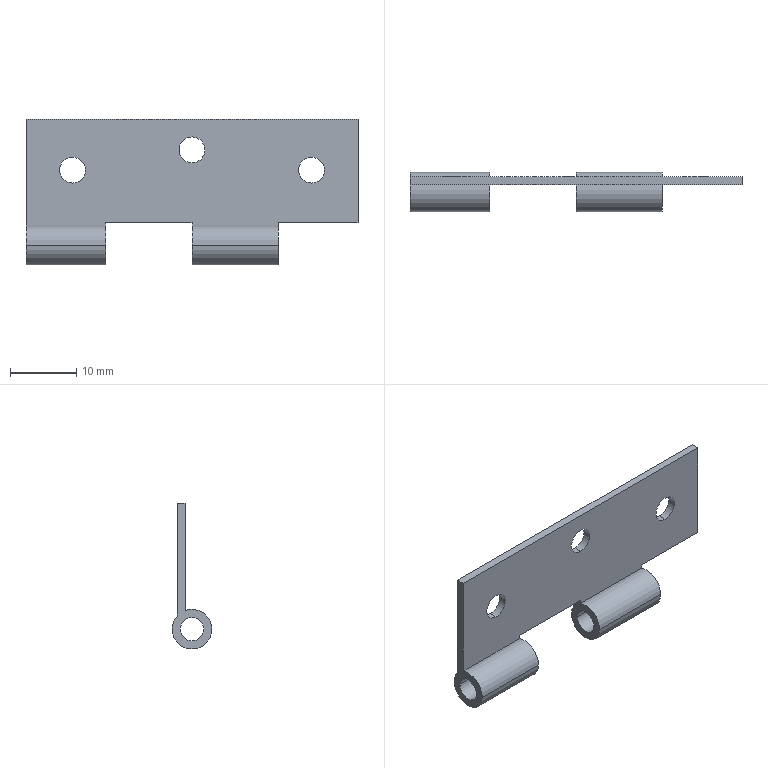Part | SolidWorks | features BaseBody 1 | 1 solid | 29 faces | box 50 x 6 x 22 mm | volume 1387 mm3 | cylinder 19 | plane 10 | commonest cylinder face diameters 3.9 x9 6 x6 3.5 x4
STEP:
#1=CARTESIAN_POINT('',(-595.131,801.497,187.232));
#2=VERTEX_POINT('',#1);
#3=CARTESIAN_POINT('',(-593.181,801.497,185.282));
#4=VERTEX_POINT('',#3);
#5=CARTESIAN_POINT('',(-595.131,801.497,185.282));
#6=DIRECTION('',(0.,1.,0.));
#7=DIRECTION('',(0.,0.,1.));
#8=AXIS2_PLACEMENT_3D('',#5,#6,#7);
#9=CIRCLE('',#8,1.95);
#10=EDGE_CURVE('',#2,#4,#9,.T.);
#11=ORIENTED_EDGE('',*,*,#10,.T.);
#12=CARTESIAN_POINT('',(-593.181,800.297,185.282));
#13=VERTEX_POINT('',#12);
#14=CARTESIAN_POINT('',(-593.181,850.297,185.282));
#15=DIRECTION('',(0.,-1.,0.));
#16=VECTOR('',#15,1000.);
#17=LINE('',#14,#16);
#18=EDGE_CURVE('',#4,#13,#17,.T.);
#19=ORIENTED_EDGE('',*,*,#18,.T.);
#20=CARTESIAN_POINT('',(-595.131,800.297,187.232));
#21=VERTEX_POINT('',#20);
#22=CARTESIAN_POINT('',(-595.131,800.297,185.282));
#23=DIRECTION('',(0.,-1.,0.));
#24=DIRECTION('',(0.,0.,-1.));
#25=AXIS2_PLACEMENT_3D('',#22,#23,#24);
#26=CIRCLE('',#25,1.95);
#27=EDGE_CURVE('',#13,#21,#26,.T.);
#28=ORIENTED_EDGE('',*,*,#27,.T.);
#29=CARTESIAN_POINT('',(-595.131,801.497,187.232));
#30=DIRECTION('',(0.,-1.,0.));
#31=VECTOR('',#30,1000.);
#32=LINE('',#29,#31);
#33=EDGE_CURVE('',#2,#21,#32,.T.);
#34=ORIENTED_EDGE('',*,*,#33,.F.);
#35=EDGE_LOOP('',(#11,#19,#28,#34));
#36=FACE_OUTER_BOUND('',#35,.T.);
#37=CARTESIAN_POINT('',(-595.131,850.297,185.282));
#38=DIRECTION('',(0.,-1.,0.));
#39=DIRECTION('',(1.,0.,0.));
#40=AXIS2_PLACEMENT_3D('',#37,#38,#39);
#41=CYLINDRICAL_SURFACE('',#40,1.95);
#42=ADVANCED_FACE('',(#36),#41,.F.);
#43=CARTESIAN_POINT('',(-631.131,801.497,187.232));
#44=VERTEX_POINT('',#43);
#45=CARTESIAN_POINT('',(-629.181,801.497,185.282));
#46=VERTEX_POINT('',#45);
#47=CARTESIAN_POINT('',(-631.131,801.497,185.282));
#48=DIRECTION('',(0.,1.,0.));
#49=DIRECTION('',(0.,0.,1.));
#50=AXIS2_PLACEMENT_3D('',#47,#48,#49);
#51=CIRCLE('',#50,1.95);
#52=EDGE_CURVE('',#44,#46,#51,.T.);
#53=ORIENTED_EDGE('',*,*,#52,.T.);
#54=CARTESIAN_POINT('',(-629.181,800.297,185.282));
#55=VERTEX_POINT('',#54);
#56=CARTESIAN_POINT('',(-629.181,850.297,185.282));
#57=DIRECTION('',(0.,-1.,0.));
#58=VECTOR('',#57,1000.);
#59=LINE('',#56,#58);
#60=EDGE_CURVE('',#46,#55,#59,.T.);
#61=ORIENTED_EDGE('',*,*,#60,.T.);
#62=CARTESIAN_POINT('',(-631.131,800.297,187.232));
#63=VERTEX_POINT('',#62);
#64=CARTESIAN_POINT('',(-631.131,800.297,185.282));
#65=DIRECTION('',(0.,-1.,0.));
#66=DIRECTION('',(0.,0.,-1.));
#67=AXIS2_PLACEMENT_3D('',#64,#65,#66);
#68=CIRCLE('',#67,1.95);
#69=EDGE_CURVE('',#55,#63,#68,.T.);
#70=ORIENTED_EDGE('',*,*,#69,.T.);
#71=CARTESIAN_POINT('',(-631.131,801.497,187.232));
#72=DIRECTION('',(0.,-1.,0.));
#73=VECTOR('',#72,1000.);
#74=LINE('',#71,#73);
#75=EDGE_CURVE('',#44,#63,#74,.T.);
#76=ORIENTED_EDGE('',*,*,#75,.F.);
#77=EDGE_LOOP('',(#53,#61,#70,#76));
#78=FACE_OUTER_BOUND('',#77,.T.);
#79=CARTESIAN_POINT('',(-631.131,850.297,185.282));
#80=DIRECTION('',(0.,-1.,0.));
#81=DIRECTION('',(1.,0.,0.));
#82=AXIS2_PLACEMENT_3D('',#79,#80,#81);
#83=CYLINDRICAL_SURFACE('',#82,1.95);
#84=ADVANCED_FACE('',(#78),#83,.F.);
#85=CARTESIAN_POINT('',(-613.131,801.497,190.282));
#86=VERTEX_POINT('',#85);
#87=CARTESIAN_POINT('',(-611.181,801.497,188.332));
#88=VERTEX_POINT('',#87);
#89=CARTESIAN_POINT('',(-613.131,801.497,188.332));
#90=DIRECTION('',(0.,1.,0.));
#91=DIRECTION('',(0.,0.,1.));
#92=AXIS2_PLACEMENT_3D('',#89,#90,#91);
#93=CIRCLE('',#92,1.95);
#94=EDGE_CURVE('',#86,#88,#93,.T.);
#95=ORIENTED_EDGE('',*,*,#94,.T.);
#96=CARTESIAN_POINT('',(-611.181,800.297,188.332));
#97=VERTEX_POINT('',#96);
#98=CARTESIAN_POINT('',(-611.181,850.297,188.332));
#99=DIRECTION('',(0.,-1.,0.));
#100=VECTOR('',#99,1000.);
#101=LINE('',#98,#100);
#102=EDGE_CURVE('',#88,#97,#101,.T.);
#103=ORIENTED_EDGE('',*,*,#102,.T.);
#104=CARTESIAN_POINT('',(-613.131,800.297,190.282));
#105=VERTEX_POINT('',#104);
#106=CARTESIAN_POINT('',(-613.131,800.297,188.332));
#107=DIRECTION('',(0.,-1.,0.));
#108=DIRECTION('',(1.,0.,0.));
#109=AXIS2_PLACEMENT_3D('',#106,#107,#108);
#110=CIRCLE('',#109,1.95);
#111=EDGE_CURVE('',#97,#105,#110,.T.);
#112=ORIENTED_EDGE('',*,*,#111,.T.);
#113=CARTESIAN_POINT('',(-613.131,800.297,190.282));
#114=DIRECTION('',(0.,1.,0.));
#115=VECTOR('',#114,1000.);
#116=LINE('',#113,#115);
#117=EDGE_CURVE('',#105,#86,#116,.T.);
#118=ORIENTED_EDGE('',*,*,#117,.T.);
#119=EDGE_LOOP('',(#95,#103,#112,#118));
#120=FACE_OUTER_BOUND('',#119,.T.);
#121=CARTESIAN_POINT('',(-613.131,850.297,188.332));
#122=DIRECTION('',(0.,-1.,0.));
#123=DIRECTION('',(1.,0.,0.));
#124=AXIS2_PLACEMENT_3D('',#121,#122,#123);
#125=CYLINDRICAL_SURFACE('',#124,1.95);
#126=ADVANCED_FACE('',(#120),#125,.F.);
#127=ORIENTED_EDGE('',*,*,#117,.F.);
#128=CARTESIAN_POINT('',(-613.131,800.297,186.382));
#129=VERTEX_POINT('',#128);
#130=CARTESIAN_POINT('',(-613.131,800.297,188.332));
#131=DIRECTION('',(0.,-1.,0.));
#132=DIRECTION('',(-1.,0.,0.));
#133=AXIS2_PLACEMENT_3D('',#130,#131,#132);
#134=CIRCLE('',#133,1.95);
#135=EDGE_CURVE('',#105,#129,#134,.T.);
#136=ORIENTED_EDGE('',*,*,#135,.T.);
#137=CARTESIAN_POINT('',(-613.131,801.497,186.382));
#138=VERTEX_POINT('',#137);
#139=CARTESIAN_POINT('',(-613.131,801.497,186.382));
#140=DIRECTION('',(0.,-1.,0.));
#141=VECTOR('',#140,1000.);
#142=LINE('',#139,#141);
#143=EDGE_CURVE('',#138,#129,#142,.T.);
#144=ORIENTED_EDGE('',*,*,#143,.F.);
#145=CARTESIAN_POINT('',(-613.131,801.497,188.332));
#146=DIRECTION('',(0.,1.,0.));
#147=DIRECTION('',(-1.,0.,0.));
#148=AXIS2_PLACEMENT_3D('',#145,#146,#147);
#149=CIRCLE('',#148,1.95);
#150=EDGE_CURVE('',#138,#86,#149,.T.);
#151=ORIENTED_EDGE('',*,*,#150,.T.);
#152=EDGE_LOOP('',(#127,#136,#144,#151));
#153=FACE_OUTER_BOUND('',#152,.T.);
#154=CARTESIAN_POINT('',(-613.131,850.297,188.332));
#155=DIRECTION('',(0.,-1.,0.));
#156=DIRECTION('',(1.,0.,0.));
#157=AXIS2_PLACEMENT_3D('',#154,#155,#156);
#158=CYLINDRICAL_SURFACE('',#157,1.95);
#159=ADVANCED_FACE('',(#153),#158,.F.);
#160=ORIENTED_EDGE('',*,*,#102,.F.);
#161=CARTESIAN_POINT('',(-613.131,801.497,188.332));
#162=DIRECTION('',(0.,1.,0.));
#163=DIRECTION('',(0.,0.,1.));
#164=AXIS2_PLACEMENT_3D('',#161,#162,#163);
#165=CIRCLE('',#164,1.95);
#166=EDGE_CURVE('',#88,#138,#165,.T.);
#167=ORIENTED_EDGE('',*,*,#166,.T.);
#168=ORIENTED_EDGE('',*,*,#143,.T.);
#169=CARTESIAN_POINT('',(-613.131,800.297,188.332));
#170=DIRECTION('',(0.,-1.,0.));
#171=DIRECTION('',(1.,0.,0.));
#172=AXIS2_PLACEMENT_3D('',#169,#170,#171);
#173=CIRCLE('',#172,1.95);
#174=EDGE_CURVE('',#129,#97,#173,.T.);
#175=ORIENTED_EDGE('',*,*,#174,.T.);
#176=EDGE_LOOP('',(#160,#167,#168,#175));
#177=FACE_OUTER_BOUND('',#176,.T.);
#178=CARTESIAN_POINT('',(-613.131,850.297,188.332));
#179=DIRECTION('',(0.,-1.,0.));
#180=DIRECTION('',(1.,0.,0.));
#181=AXIS2_PLACEMENT_3D('',#178,#179,#180);
#182=CYLINDRICAL_SURFACE('',#181,1.95);
#183=ADVANCED_FACE('',(#177),#182,.F.);
#184=CARTESIAN_POINT('',(-626.131,801.497,175.966));
#185=VERTEX_POINT('',#184);
#186=CARTESIAN_POINT('',(-626.131,801.497,177.382));
#187=VERTEX_POINT('',#186);
#188=CARTESIAN_POINT('',(-626.131,801.497,175.966));
#189=DIRECTION('',(0.,0.,1.));
#190=VECTOR('',#189,1000.);
#191=LINE('',#188,#190);
#192=EDGE_CURVE('',#185,#187,#191,.T.);
#193=ORIENTED_EDGE('',*,*,#192,.F.);
#194=CARTESIAN_POINT('',(-638.131,801.497,175.966));
#195=VERTEX_POINT('',#194);
#196=CARTESIAN_POINT('',(-626.131,801.497,175.966));
#197=DIRECTION('',(-1.,0.,0.));
#198=VECTOR('',#197,1000.);
#199=LINE('',#196,#198);
#200=EDGE_CURVE('',#185,#195,#199,.T.);
#201=ORIENTED_EDGE('',*,*,#200,.T.);
#202=CARTESIAN_POINT('',(-638.131,801.497,192.982));
#203=VERTEX_POINT('',#202);
#204=CARTESIAN_POINT('',(-638.131,801.497,192.982));
#205=DIRECTION('',(0.,0.,-1.));
#206=VECTOR('',#205,1000.);
#207=LINE('',#204,#206);
#208=EDGE_CURVE('',#203,#195,#207,.T.);
#209=ORIENTED_EDGE('',*,*,#208,.F.);
#210=CARTESIAN_POINT('',(-588.131,801.497,192.982));
#211=VERTEX_POINT('',#210);
#212=CARTESIAN_POINT('',(-588.131,801.497,192.982));
#213=DIRECTION('',(-1.,0.,0.));
#214=VECTOR('',#213,1000.);
#215=LINE('',#212,#214);
#216=EDGE_CURVE('',#211,#203,#215,.T.);
#217=ORIENTED_EDGE('',*,*,#216,.F.);
#218=CARTESIAN_POINT('',(-588.131,801.497,177.382));
#219=VERTEX_POINT('',#218);
#220=CARTESIAN_POINT('',(-588.131,801.497,177.382));
#221=DIRECTION('',(0.,0.,1.));
#222=VECTOR('',#221,1000.);
#223=LINE('',#220,#222);
#224=EDGE_CURVE('',#219,#211,#223,.T.);
#225=ORIENTED_EDGE('',*,*,#224,.F.);
#226=CARTESIAN_POINT('',(-600.131,801.497,177.382));
#227=VERTEX_POINT('',#226);
#228=CARTESIAN_POINT('',(-600.131,801.497,177.382));
#229=DIRECTION('',(1.,0.,0.));
#230=VECTOR('',#229,1000.);
#231=LINE('',#228,#230);
#232=EDGE_CURVE('',#227,#219,#231,.T.);
#233=ORIENTED_EDGE('',*,*,#232,.F.);
#234=CARTESIAN_POINT('',(-600.131,801.497,175.966));
#235=VERTEX_POINT('',#234);
#236=CARTESIAN_POINT('',(-600.131,801.497,175.966));
#237=DIRECTION('',(0.,0.,1.));
#238=VECTOR('',#237,1000.);
#239=LINE('',#236,#238);
#240=EDGE_CURVE('',#235,#227,#239,.T.);
#241=ORIENTED_EDGE('',*,*,#240,.F.);
#242=CARTESIAN_POINT('',(-613.131,801.497,175.966));
#243=VERTEX_POINT('',#242);
#244=CARTESIAN_POINT('',(-600.131,801.497,175.966));
#245=DIRECTION('',(-1.,0.,0.));
#246=VECTOR('',#245,1000.);
#247=LINE('',#244,#246);
#248=EDGE_CURVE('',#235,#243,#247,.T.);
#249=ORIENTED_EDGE('',*,*,#248,.T.);
#250=CARTESIAN_POINT('',(-613.131,801.497,177.382));
#251=VERTEX_POINT('',#250);
#252=CARTESIAN_POINT('',(-613.131,801.497,177.382));
#253=DIRECTION('',(0.,0.,-1.));
#254=VECTOR('',#253,1000.);
#255=LINE('',#252,#254);
#256=EDGE_CURVE('',#251,#243,#255,.T.);
#257=ORIENTED_EDGE('',*,*,#256,.F.);
#258=CARTESIAN_POINT('',(-626.131,801.497,177.382));
#259=DIRECTION('',(1.,0.,0.));
#260=VECTOR('',#259,1000.);
#261=LINE('',#258,#260);
#262=EDGE_CURVE('',#187,#251,#261,.T.);
#263=ORIENTED_EDGE('',*,*,#262,.F.);
#264=EDGE_LOOP('',(#193,#201,#209,#217,#225,#233,#241,#249,#257,#263));
#265=FACE_OUTER_BOUND('',#264,.T.);
#266=ORIENTED_EDGE('',*,*,#150,.F.);
#267=ORIENTED_EDGE('',*,*,#166,.F.);
#268=ORIENTED_EDGE('',*,*,#94,.F.);
#269=EDGE_LOOP('',(#266,#267,#268));
#270=FACE_BOUND('',#269,.T.);
#271=CARTESIAN_POINT('',(-631.131,801.497,183.332));
#272=VERTEX_POINT('',#271);
#273=CARTESIAN_POINT('',(-631.131,801.497,185.282));
#274=DIRECTION('',(0.,1.,0.));
#275=DIRECTION('',(-1.,0.,0.));
#276=AXIS2_PLACEMENT_3D('',#273,#274,#275);
#277=CIRCLE('',#276,1.95);
#278=EDGE_CURVE('',#272,#44,#277,.T.);
#279=ORIENTED_EDGE('',*,*,#278,.F.);
#280=CARTESIAN_POINT('',(-631.131,801.497,185.282));
#281=DIRECTION('',(0.,1.,0.));
#282=DIRECTION('',(0.,0.,1.));
#283=AXIS2_PLACEMENT_3D('',#280,#281,#282);
#284=CIRCLE('',#283,1.95);
#285=EDGE_CURVE('',#46,#272,#284,.T.);
#286=ORIENTED_EDGE('',*,*,#285,.F.);
#287=ORIENTED_EDGE('',*,*,#52,.F.);
#288=EDGE_LOOP('',(#279,#286,#287));
#289=FACE_BOUND('',#288,.T.);
#290=CARTESIAN_POINT('',(-595.131,801.497,183.332));
#291=VERTEX_POINT('',#290);
#292=CARTESIAN_POINT('',(-595.131,801.497,185.282));
#293=DIRECTION('',(0.,1.,0.));
#294=DIRECTION('',(-1.,0.,0.));
#295=AXIS2_PLACEMENT_3D('',#292,#293,#294);
#296=CIRCLE('',#295,1.95);
#297=EDGE_CURVE('',#291,#2,#296,.T.);
#298=ORIENTED_EDGE('',*,*,#297,.F.);
#299=CARTESIAN_POINT('',(-595.131,801.497,185.282));
#300=DIRECTION('',(0.,1.,0.));
#301=DIRECTION('',(0.,0.,1.));
#302=AXIS2_PLACEMENT_3D('',#299,#300,#301);
#303=CIRCLE('',#302,1.95);
#304=EDGE_CURVE('',#4,#291,#303,.T.);
#305=ORIENTED_EDGE('',*,*,#304,.F.);
#306=ORIENTED_EDGE('',*,*,#10,.F.);
#307=EDGE_LOOP('',(#298,#305,#306));
#308=FACE_BOUND('',#307,.T.);
#309=CARTESIAN_POINT('',(-588.131,801.497,175.966));
#310=DIRECTION('',(0.,-1.,0.));
#311=DIRECTION('',(0.,0.,1.));
#312=AXIS2_PLACEMENT_3D('',#309,#310,#311);
#313=PLANE('',#312);
#314=ADVANCED_FACE('',(#265,#270,#289,#308),#313,.F.);
#315=ORIENTED_EDGE('',*,*,#262,.T.);
#316=CARTESIAN_POINT('',(-613.131,800.297,177.382));
#317=VERTEX_POINT('',#316);
#318=CARTESIAN_POINT('',(-613.131,801.497,177.382));
#319=DIRECTION('',(0.,-1.,0.));
#320=VECTOR('',#319,1000.);
#321=LINE('',#318,#320);
#322=EDGE_CURVE('',#251,#317,#321,.T.);
#323=ORIENTED_EDGE('',*,*,#322,.T.);
#324=CARTESIAN_POINT('',(-626.131,800.297,177.382));
#325=VERTEX_POINT('',#324);
#326=CARTESIAN_POINT('',(-613.131,800.297,177.382));
#327=DIRECTION('',(-1.,0.,0.));
#328=VECTOR('',#327,1000.);
#329=LINE('',#326,#328);
#330=EDGE_CURVE('',#317,#325,#329,.T.);
#331=ORIENTED_EDGE('',*,*,#330,.T.);
#332=CARTESIAN_POINT('',(-626.131,801.497,177.382));
#333=DIRECTION('',(0.,-1.,0.));
#334=VECTOR('',#333,1000.);
#335=LINE('',#332,#334);
#336=EDGE_CURVE('',#187,#325,#335,.T.);
#337=ORIENTED_EDGE('',*,*,#336,.F.);
#338=EDGE_LOOP('',(#315,#323,#331,#337));
#339=FACE_OUTER_BOUND('',#338,.T.);
#340=CARTESIAN_POINT('',(-613.131,750.297,177.382));
#341=DIRECTION('',(0.,0.,-1.));
#342=DIRECTION('',(0.,-1.,0.));
#343=AXIS2_PLACEMENT_3D('',#340,#341,#342);
#344=PLANE('',#343);
#345=ADVANCED_FACE('',(#339),#344,.T.);
#346=CARTESIAN_POINT('',(-626.131,802.247,173.982));
#347=VERTEX_POINT('',#346);
#348=CARTESIAN_POINT('',(-626.131,796.247,173.982));
#349=VERTEX_POINT('',#348);
#350=CARTESIAN_POINT('',(-626.131,799.247,173.982));
#351=DIRECTION('',(-1.,0.,0.));
#352=DIRECTION('',(0.,1.,0.));
#353=AXIS2_PLACEMENT_3D('',#350,#351,#352);
#354=CIRCLE('',#353,3.);
#355=EDGE_CURVE('',#347,#349,#354,.T.);
#356=ORIENTED_EDGE('',*,*,#355,.F.);
#357=CARTESIAN_POINT('',(-626.131,799.247,173.982));
#358=DIRECTION('',(-1.,0.,0.));
#359=DIRECTION('',(0.,0.75,0.6614));
#360=AXIS2_PLACEMENT_3D('',#357,#358,#359);
#361=CIRCLE('',#360,3.);
#362=EDGE_CURVE('',#185,#347,#361,.T.);
#363=ORIENTED_EDGE('',*,*,#362,.F.);
#364=ORIENTED_EDGE('',*,*,#192,.T.);
#365=ORIENTED_EDGE('',*,*,#336,.T.);
#366=CARTESIAN_POINT('',(-626.131,800.297,176.792));
#367=VERTEX_POINT('',#366);
#368=CARTESIAN_POINT('',(-626.131,800.297,177.382));
#369=DIRECTION('',(0.,0.,-1.));
#370=VECTOR('',#369,1000.);
#371=LINE('',#368,#370);
#372=EDGE_CURVE('',#325,#367,#371,.T.);
#373=ORIENTED_EDGE('',*,*,#372,.T.);
#374=CARTESIAN_POINT('',(-626.131,799.247,173.982));
#375=DIRECTION('',(-1.,0.,0.));
#376=DIRECTION('',(0.,-1.,0.));
#377=AXIS2_PLACEMENT_3D('',#374,#375,#376);
#378=CIRCLE('',#377,3.);
#379=EDGE_CURVE('',#349,#367,#378,.T.);
#380=ORIENTED_EDGE('',*,*,#379,.F.);
#381=EDGE_LOOP('',(#356,#363,#364,#365,#373,#380));
#382=FACE_OUTER_BOUND('',#381,.T.);
#383=CARTESIAN_POINT('',(-626.131,800.997,173.982));
#384=VERTEX_POINT('',#383);
#385=CARTESIAN_POINT('',(-626.131,797.497,173.982));
#386=VERTEX_POINT('',#385);
#387=CARTESIAN_POINT('',(-626.131,799.247,173.982));
#388=DIRECTION('',(1.,0.,0.));
#389=DIRECTION('',(0.,1.,0.));
#390=AXIS2_PLACEMENT_3D('',#387,#388,#389);
#391=CIRCLE('',#390,1.75);
#392=EDGE_CURVE('',#384,#386,#391,.T.);
#393=ORIENTED_EDGE('',*,*,#392,.F.);
#394=CARTESIAN_POINT('',(-626.131,799.247,173.982));
#395=DIRECTION('',(1.,0.,0.));
#396=DIRECTION('',(0.,-1.,0.));
#397=AXIS2_PLACEMENT_3D('',#394,#395,#396);
#398=CIRCLE('',#397,1.75);
#399=EDGE_CURVE('',#386,#384,#398,.T.);
#400=ORIENTED_EDGE('',*,*,#399,.F.);
#401=EDGE_LOOP('',(#393,#400));
#402=FACE_BOUND('',#401,.T.);
#403=CARTESIAN_POINT('',(-626.131,750.297,177.382));
#404=DIRECTION('',(1.,0.,0.));
#405=DIRECTION('',(0.,1.,0.));
#406=AXIS2_PLACEMENT_3D('',#403,#404,#405);
#407=PLANE('',#406);
#408=ADVANCED_FACE('',(#382,#402),#407,.T.);
#409=CARTESIAN_POINT('',(-638.131,800.297,176.792));
#410=VERTEX_POINT('',#409);
#411=CARTESIAN_POINT('',(-638.131,800.297,176.792));
#412=DIRECTION('',(1.,0.,0.));
#413=VECTOR('',#412,1000.);
#414=LINE('',#411,#413);
#415=EDGE_CURVE('',#410,#367,#414,.T.);
#416=ORIENTED_EDGE('',*,*,#415,.F.);
#417=CARTESIAN_POINT('',(-638.131,796.247,173.982));
#418=VERTEX_POINT('',#417);
#419=CARTESIAN_POINT('',(-638.131,799.247,173.982));
#420=DIRECTION('',(1.,0.,0.));
#421=DIRECTION('',(0.,0.35,0.9367));
#422=AXIS2_PLACEMENT_3D('',#419,#420,#421);
#423=CIRCLE('',#422,3.);
#424=EDGE_CURVE('',#410,#418,#423,.T.);
#425=ORIENTED_EDGE('',*,*,#424,.T.);
#426=CARTESIAN_POINT('',(-626.131,796.247,173.982));
#427=DIRECTION('',(-1.,0.,0.));
#428=VECTOR('',#427,1000.);
#429=LINE('',#426,#428);
#430=EDGE_CURVE('',#349,#418,#429,.T.);
#431=ORIENTED_EDGE('',*,*,#430,.F.);
#432=ORIENTED_EDGE('',*,*,#379,.T.);
#433=EDGE_LOOP('',(#416,#425,#431,#432));
#434=FACE_OUTER_BOUND('',#433,.T.);
#435=CARTESIAN_POINT('',(-588.131,799.247,173.982));
#436=DIRECTION('',(-1.,0.,0.));
#437=DIRECTION('',(0.,-1.,0.));
#438=AXIS2_PLACEMENT_3D('',#435,#436,#437);
#439=CYLINDRICAL_SURFACE('',#438,3.);
#440=ADVANCED_FACE('',(#434),#439,.T.);
#441=CARTESIAN_POINT('',(-638.131,802.247,173.982));
#442=VERTEX_POINT('',#441);
#443=CARTESIAN_POINT('',(-638.131,799.247,173.982));
#444=DIRECTION('',(1.,0.,0.));
#445=DIRECTION('',(0.,-1.,0.));
#446=AXIS2_PLACEMENT_3D('',#443,#444,#445);
#447=CIRCLE('',#446,3.);
#448=EDGE_CURVE('',#418,#442,#447,.T.);
#449=ORIENTED_EDGE('',*,*,#448,.T.);
#450=CARTESIAN_POINT('',(-638.131,802.247,173.982));
#451=DIRECTION('',(1.,0.,0.));
#452=VECTOR('',#451,1000.);
#453=LINE('',#450,#452);
#454=EDGE_CURVE('',#442,#347,#453,.T.);
#455=ORIENTED_EDGE('',*,*,#454,.T.);
#456=ORIENTED_EDGE('',*,*,#355,.T.);
#457=ORIENTED_EDGE('',*,*,#430,.T.);
#458=EDGE_LOOP('',(#449,#455,#456,#457));
#459=FACE_OUTER_BOUND('',#458,.T.);
#460=CARTESIAN_POINT('',(-588.131,799.247,173.982));
#461=DIRECTION('',(-1.,0.,0.));
#462=DIRECTION('',(0.,-1.,0.));
#463=AXIS2_PLACEMENT_3D('',#460,#461,#462);
#464=CYLINDRICAL_SURFACE('',#463,3.);
#465=ADVANCED_FACE('',(#459),#464,.T.);
#466=CARTESIAN_POINT('',(-638.131,799.247,173.982));
#467=DIRECTION('',(1.,0.,0.));
#468=DIRECTION('',(0.,1.,0.));
#469=AXIS2_PLACEMENT_3D('',#466,#467,#468);
#470=CIRCLE('',#469,3.);
#471=EDGE_CURVE('',#442,#195,#470,.T.);
#472=ORIENTED_EDGE('',*,*,#471,.T.);
#473=ORIENTED_EDGE('',*,*,#200,.F.);
#474=ORIENTED_EDGE('',*,*,#362,.T.);
#475=ORIENTED_EDGE('',*,*,#454,.F.);
#476=EDGE_LOOP('',(#472,#473,#474,#475));
#477=FACE_OUTER_BOUND('',#476,.T.);
#478=CARTESIAN_POINT('',(-588.131,799.247,173.982));
#479=DIRECTION('',(-1.,0.,0.));
#480=DIRECTION('',(0.,-1.,0.));
#481=AXIS2_PLACEMENT_3D('',#478,#479,#480);
#482=CYLINDRICAL_SURFACE('',#481,3.);
#483=ADVANCED_FACE('',(#477),#482,.T.);
#484=ORIENTED_EDGE('',*,*,#208,.T.);
#485=ORIENTED_EDGE('',*,*,#471,.F.);
#486=ORIENTED_EDGE('',*,*,#448,.F.);
#487=ORIENTED_EDGE('',*,*,#424,.F.);
#488=CARTESIAN_POINT('',(-638.131,800.297,192.982));
#489=VERTEX_POINT('',#488);
#490=CARTESIAN_POINT('',(-638.131,800.297,176.792));
#491=DIRECTION('',(0.,0.,1.));
#492=VECTOR('',#491,1000.);
#493=LINE('',#490,#492);
#494=EDGE_CURVE('',#410,#489,#493,.T.);
#495=ORIENTED_EDGE('',*,*,#494,.T.);
#496=CARTESIAN_POINT('',(-638.131,801.497,192.982));
#497=DIRECTION('',(0.,-1.,0.));
#498=VECTOR('',#497,1000.);
#499=LINE('',#496,#498);
#500=EDGE_CURVE('',#203,#489,#499,.T.);
#501=ORIENTED_EDGE('',*,*,#500,.F.);
#502=EDGE_LOOP('',(#484,#485,#486,#487,#495,#501));
#503=FACE_OUTER_BOUND('',#502,.T.);
#504=CARTESIAN_POINT('',(-638.131,800.997,173.982));
#505=VERTEX_POINT('',#504);
#506=CARTESIAN_POINT('',(-638.131,797.497,173.982));
#507=VERTEX_POINT('',#506);
#508=CARTESIAN_POINT('',(-638.131,799.247,173.982));
#509=DIRECTION('',(-1.,0.,0.));
#510=DIRECTION('',(0.,1.,0.));
#511=AXIS2_PLACEMENT_3D('',#508,#509,#510);
#512=CIRCLE('',#511,1.75);
#513=EDGE_CURVE('',#505,#507,#512,.T.);
#514=ORIENTED_EDGE('',*,*,#513,.F.);
#515=CARTESIAN_POINT('',(-638.131,799.247,173.982));
#516=DIRECTION('',(-1.,0.,0.));
#517=DIRECTION('',(0.,-1.,0.));
#518=AXIS2_PLACEMENT_3D('',#515,#516,#517);
#519=CIRCLE('',#518,1.75);
#520=EDGE_CURVE('',#507,#505,#519,.T.);
#521=ORIENTED_EDGE('',*,*,#520,.F.);
#522=EDGE_LOOP('',(#514,#521));
#523=FACE_BOUND('',#522,.T.);
#524=CARTESIAN_POINT('',(-638.131,799.247,173.982));
#525=DIRECTION('',(1.,0.,0.));
#526=DIRECTION('',(0.,1.,0.));
#527=AXIS2_PLACEMENT_3D('',#524,#525,#526);
#528=PLANE('',#527);
#529=ADVANCED_FACE('',(#503,#523),#528,.F.);
#530=CARTESIAN_POINT('',(-588.131,800.297,192.982));
#531=VERTEX_POINT('',#530);
#532=CARTESIAN_POINT('',(-588.131,801.497,192.982));
#533=DIRECTION('',(0.,-1.,0.));
#534=VECTOR('',#533,1000.);
#535=LINE('',#532,#534);
#536=EDGE_CURVE('',#211,#531,#535,.T.);
#537=ORIENTED_EDGE('',*,*,#536,.F.);
#538=ORIENTED_EDGE('',*,*,#216,.T.);
#539=ORIENTED_EDGE('',*,*,#500,.T.);
#540=CARTESIAN_POINT('',(-638.131,800.297,192.982));
#541=DIRECTION('',(1.,0.,0.));
#542=VECTOR('',#541,1000.);
#543=LINE('',#540,#542);
#544=EDGE_CURVE('',#489,#531,#543,.T.);
#545=ORIENTED_EDGE('',*,*,#544,.T.);
#546=EDGE_LOOP('',(#537,#538,#539,#545));
#547=FACE_OUTER_BOUND('',#546,.T.);
#548=CARTESIAN_POINT('',(-588.131,801.497,192.982));
#549=DIRECTION('',(0.,0.,-1.));
#550=DIRECTION('',(-1.,0.,0.));
#551=AXIS2_PLACEMENT_3D('',#548,#549,#550);
#552=PLANE('',#551);
#553=ADVANCED_FACE('',(#547),#552,.F.);
#554=CARTESIAN_POINT('',(-600.131,800.297,177.382));
#555=VERTEX_POINT('',#554);
#556=CARTESIAN_POINT('',(-600.131,800.297,176.792));
#557=VERTEX_POINT('',#556);
#558=CARTESIAN_POINT('',(-600.131,800.297,177.382));
#559=DIRECTION('',(0.,0.,-1.));
#560=VECTOR('',#559,1000.);
#561=LINE('',#558,#560);
#562=EDGE_CURVE('',#555,#557,#561,.T.);
#563=ORIENTED_EDGE('',*,*,#562,.F.);
#564=CARTESIAN_POINT('',(-588.131,800.297,177.382));
#565=VERTEX_POINT('',#564);
#566=CARTESIAN_POINT('',(-588.131,800.297,177.382));
#567=DIRECTION('',(-1.,0.,0.));
#568=VECTOR('',#567,1000.);
#569=LINE('',#566,#568);
#570=EDGE_CURVE('',#565,#555,#569,.T.);
#571=ORIENTED_EDGE('',*,*,#570,.F.);
#572=CARTESIAN_POINT('',(-588.131,800.297,192.982));
#573=DIRECTION('',(0.,0.,-1.));
#574=VECTOR('',#573,1000.);
#575=LINE('',#572,#574);
#576=EDGE_CURVE('',#531,#565,#575,.T.);
#577=ORIENTED_EDGE('',*,*,#576,.F.);
#578=ORIENTED_EDGE('',*,*,#544,.F.);
#579=ORIENTED_EDGE('',*,*,#494,.F.);
#580=ORIENTED_EDGE('',*,*,#415,.T.);
#581=ORIENTED_EDGE('',*,*,#372,.F.);
#582=ORIENTED_EDGE('',*,*,#330,.F.);
#583=CARTESIAN_POINT('',(-613.131,800.297,176.792));
#584=VERTEX_POINT('',#583);
#585=CARTESIAN_POINT('',(-613.131,800.297,177.382));
#586=DIRECTION('',(0.,0.,-1.));
#587=VECTOR('',#586,1000.);
#588=LINE('',#585,#587);
#589=EDGE_CURVE('',#317,#584,#588,.T.);
#590=ORIENTED_EDGE('',*,*,#589,.T.);
#591=CARTESIAN_POINT('',(-613.131,800.297,176.792));
#592=DIRECTION('',(1.,0.,0.));
#593=VECTOR('',#592,1000.);
#594=LINE('',#591,#593);
#595=EDGE_CURVE('',#584,#557,#594,.T.);
#596=ORIENTED_EDGE('',*,*,#595,.T.);
#597=EDGE_LOOP('',(#563,#571,#577,#578,#579,#580,#581,#582,#590,#596));
#598=FACE_OUTER_BOUND('',#597,.T.);
#599=ORIENTED_EDGE('',*,*,#135,.F.);
#600=ORIENTED_EDGE('',*,*,#111,.F.);
#601=ORIENTED_EDGE('',*,*,#174,.F.);
#602=EDGE_LOOP('',(#599,#600,#601));
#603=FACE_BOUND('',#602,.T.);
#604=CARTESIAN_POINT('',(-631.131,800.297,183.332));
#605=VERTEX_POINT('',#604);
#606=CARTESIAN_POINT('',(-631.131,800.297,185.282));
#607=DIRECTION('',(0.,-1.,0.));
#608=DIRECTION('',(-1.,0.,0.));
#609=AXIS2_PLACEMENT_3D('',#606,#607,#608);
#610=CIRCLE('',#609,1.95);
#611=EDGE_CURVE('',#63,#605,#610,.T.);
#612=ORIENTED_EDGE('',*,*,#611,.F.);
#613=ORIENTED_EDGE('',*,*,#69,.F.);
#614=CARTESIAN_POINT('',(-631.131,800.297,185.282));
#615=DIRECTION('',(0.,-1.,0.));
#616=DIRECTION('',(0.,0.,-1.));
#617=AXIS2_PLACEMENT_3D('',#614,#615,#616);
#618=CIRCLE('',#617,1.95);
#619=EDGE_CURVE('',#605,#55,#618,.T.);
#620=ORIENTED_EDGE('',*,*,#619,.F.);
#621=EDGE_LOOP('',(#612,#613,#620));
#622=FACE_BOUND('',#621,.T.);
#623=CARTESIAN_POINT('',(-595.131,800.297,183.332));
#624=VERTEX_POINT('',#623);
#625=CARTESIAN_POINT('',(-595.131,800.297,185.282));
#626=DIRECTION('',(0.,-1.,0.));
#627=DIRECTION('',(-1.,0.,0.));
#628=AXIS2_PLACEMENT_3D('',#625,#626,#627);
#629=CIRCLE('',#628,1.95);
#630=EDGE_CURVE('',#21,#624,#629,.T.);
#631=ORIENTED_EDGE('',*,*,#630,.F.);
#632=ORIENTED_EDGE('',*,*,#27,.F.);
#633=CARTESIAN_POINT('',(-595.131,800.297,185.282));
#634=DIRECTION('',(0.,-1.,0.));
#635=DIRECTION('',(0.,0.,-1.));
#636=AXIS2_PLACEMENT_3D('',#633,#634,#635);
#637=CIRCLE('',#636,1.95);
#638=EDGE_CURVE('',#624,#13,#637,.T.);
#639=ORIENTED_EDGE('',*,*,#638,.F.);
#640=EDGE_LOOP('',(#631,#632,#639));
#641=FACE_BOUND('',#640,.T.);
#642=CARTESIAN_POINT('',(-588.131,800.297,176.792));
#643=DIRECTION('',(0.,1.,0.));
#644=DIRECTION('',(0.,0.,-1.));
#645=AXIS2_PLACEMENT_3D('',#642,#643,#644);
#646=PLANE('',#645);
#647=ADVANCED_FACE('',(#598,#603,#622,#641),#646,.F.);
#648=ORIENTED_EDGE('',*,*,#595,.F.);
#649=CARTESIAN_POINT('',(-613.131,796.247,173.982));
#650=VERTEX_POINT('',#649);
#651=CARTESIAN_POINT('',(-613.131,799.247,173.982));
#652=DIRECTION('',(1.,0.,0.));
#653=DIRECTION('',(0.,0.35,0.9367));
#654=AXIS2_PLACEMENT_3D('',#651,#652,#653);
#655=CIRCLE('',#654,3.);
#656=EDGE_CURVE('',#584,#650,#655,.T.);
#657=ORIENTED_EDGE('',*,*,#656,.T.);
#658=CARTESIAN_POINT('',(-600.131,796.247,173.982));
#659=VERTEX_POINT('',#658);
#660=CARTESIAN_POINT('',(-613.131,796.247,173.982));
#661=DIRECTION('',(1.,0.,0.));
#662=VECTOR('',#661,1000.);
#663=LINE('',#660,#662);
#664=EDGE_CURVE('',#650,#659,#663,.T.);
#665=ORIENTED_EDGE('',*,*,#664,.T.);
#666=CARTESIAN_POINT('',(-600.131,799.247,173.982));
#667=DIRECTION('',(-1.,0.,0.));
#668=DIRECTION('',(0.,-1.,0.));
#669=AXIS2_PLACEMENT_3D('',#666,#667,#668);
#670=CIRCLE('',#669,3.);
#671=EDGE_CURVE('',#659,#557,#670,.T.);
#672=ORIENTED_EDGE('',*,*,#671,.T.);
#673=EDGE_LOOP('',(#648,#657,#665,#672));
#674=FACE_OUTER_BOUND('',#673,.T.);
#675=CARTESIAN_POINT('',(-588.131,799.247,173.982));
#676=DIRECTION('',(-1.,0.,0.));
#677=DIRECTION('',(0.,-1.,0.));
#678=AXIS2_PLACEMENT_3D('',#675,#676,#677);
#679=CYLINDRICAL_SURFACE('',#678,3.);
#680=ADVANCED_FACE('',(#674),#679,.T.);
#681=CARTESIAN_POINT('',(-600.131,802.247,173.982));
#682=VERTEX_POINT('',#681);
#683=CARTESIAN_POINT('',(-600.131,799.247,173.982));
#684=DIRECTION('',(-1.,0.,0.));
#685=DIRECTION('',(0.,1.,0.));
#686=AXIS2_PLACEMENT_3D('',#683,#684,#685);
#687=CIRCLE('',#686,3.);
#688=EDGE_CURVE('',#682,#659,#687,.T.);
#689=ORIENTED_EDGE('',*,*,#688,.F.);
#690=CARTESIAN_POINT('',(-600.131,799.247,173.982));
#691=DIRECTION('',(-1.,0.,0.));
#692=DIRECTION('',(0.,0.75,0.6614));
#693=AXIS2_PLACEMENT_3D('',#690,#691,#692);
#694=CIRCLE('',#693,3.);
#695=EDGE_CURVE('',#235,#682,#694,.T.);
#696=ORIENTED_EDGE('',*,*,#695,.F.);
#697=ORIENTED_EDGE('',*,*,#240,.T.);
#698=CARTESIAN_POINT('',(-600.131,801.497,177.382));
#699=DIRECTION('',(0.,-1.,0.));
#700=VECTOR('',#699,1000.);
#701=LINE('',#698,#700);
#702=EDGE_CURVE('',#227,#555,#701,.T.);
#703=ORIENTED_EDGE('',*,*,#702,.T.);
#704=ORIENTED_EDGE('',*,*,#562,.T.);
#705=ORIENTED_EDGE('',*,*,#671,.F.);
#706=EDGE_LOOP('',(#689,#696,#697,#703,#704,#705));
#707=FACE_OUTER_BOUND('',#706,.T.);
#708=CARTESIAN_POINT('',(-600.131,800.997,173.982));
#709=VERTEX_POINT('',#708);
#710=CARTESIAN_POINT('',(-600.131,797.497,173.982));
#711=VERTEX_POINT('',#710);
#712=CARTESIAN_POINT('',(-600.131,799.247,173.982));
#713=DIRECTION('',(1.,0.,0.));
#714=DIRECTION('',(0.,1.,0.));
#715=AXIS2_PLACEMENT_3D('',#712,#713,#714);
#716=CIRCLE('',#715,1.75);
#717=EDGE_CURVE('',#709,#711,#716,.T.);
#718=ORIENTED_EDGE('',*,*,#717,.F.);
#719=CARTESIAN_POINT('',(-600.131,799.247,173.982));
#720=DIRECTION('',(1.,0.,0.));
#721=DIRECTION('',(0.,-1.,0.));
#722=AXIS2_PLACEMENT_3D('',#719,#720,#721);
#723=CIRCLE('',#722,1.75);
#724=EDGE_CURVE('',#711,#709,#723,.T.);
#725=ORIENTED_EDGE('',*,*,#724,.F.);
#726=EDGE_LOOP('',(#718,#725));
#727=FACE_BOUND('',#726,.T.);
#728=CARTESIAN_POINT('',(-600.131,750.297,165.604));
#729=DIRECTION('',(1.,0.,0.));
#730=DIRECTION('',(0.,1.,0.));
#731=AXIS2_PLACEMENT_3D('',#728,#729,#730);
#732=PLANE('',#731);
#733=ADVANCED_FACE('',(#707,#727),#732,.T.);
#734=ORIENTED_EDGE('',*,*,#232,.T.);
#735=CARTESIAN_POINT('',(-588.131,801.497,177.382));
#736=DIRECTION('',(0.,-1.,0.));
#737=VECTOR('',#736,1000.);
#738=LINE('',#735,#737);
#739=EDGE_CURVE('',#219,#565,#738,.T.);
#740=ORIENTED_EDGE('',*,*,#739,.T.);
#741=ORIENTED_EDGE('',*,*,#570,.T.);
#742=ORIENTED_EDGE('',*,*,#702,.F.);
#743=EDGE_LOOP('',(#734,#740,#741,#742));
#744=FACE_OUTER_BOUND('',#743,.T.);
#745=CARTESIAN_POINT('',(-583.249,750.297,177.382));
#746=DIRECTION('',(0.,0.,-1.));
#747=DIRECTION('',(0.,-1.,0.));
#748=AXIS2_PLACEMENT_3D('',#745,#746,#747);
#749=PLANE('',#748);
#750=ADVANCED_FACE('',(#744),#749,.T.);
#751=ORIENTED_EDGE('',*,*,#224,.T.);
#752=ORIENTED_EDGE('',*,*,#536,.T.);
#753=ORIENTED_EDGE('',*,*,#576,.T.);
#754=ORIENTED_EDGE('',*,*,#739,.F.);
#755=EDGE_LOOP('',(#751,#752,#753,#754));
#756=FACE_OUTER_BOUND('',#755,.T.);
#757=CARTESIAN_POINT('',(-588.131,799.247,173.982));
#758=DIRECTION('',(1.,0.,0.));
#759=DIRECTION('',(0.,1.,0.));
#760=AXIS2_PLACEMENT_3D('',#757,#758,#759);
#761=PLANE('',#760);
#762=ADVANCED_FACE('',(#756),#761,.T.);
#763=CARTESIAN_POINT('',(-613.131,802.247,173.982));
#764=VERTEX_POINT('',#763);
#765=CARTESIAN_POINT('',(-613.131,799.247,173.982));
#766=DIRECTION('',(1.,0.,0.));
#767=DIRECTION('',(0.,1.,0.));
#768=AXIS2_PLACEMENT_3D('',#765,#766,#767);
#769=CIRCLE('',#768,3.);
#770=EDGE_CURVE('',#764,#243,#769,.T.);
#771=ORIENTED_EDGE('',*,*,#770,.T.);
#772=ORIENTED_EDGE('',*,*,#248,.F.);
#773=ORIENTED_EDGE('',*,*,#695,.T.);
#774=CARTESIAN_POINT('',(-613.131,802.247,173.982));
#775=DIRECTION('',(1.,0.,0.));
#776=VECTOR('',#775,1000.);
#777=LINE('',#774,#776);
#778=EDGE_CURVE('',#764,#682,#777,.T.);
#779=ORIENTED_EDGE('',*,*,#778,.F.);
#780=EDGE_LOOP('',(#771,#772,#773,#779));
#781=FACE_OUTER_BOUND('',#780,.T.);
#782=CARTESIAN_POINT('',(-588.131,799.247,173.982));
#783=DIRECTION('',(-1.,0.,0.));
#784=DIRECTION('',(0.,-1.,0.));
#785=AXIS2_PLACEMENT_3D('',#782,#783,#784);
#786=CYLINDRICAL_SURFACE('',#785,3.);
#787=ADVANCED_FACE('',(#781),#786,.T.);
#788=CARTESIAN_POINT('',(-613.131,799.247,173.982));
#789=DIRECTION('',(1.,0.,0.));
#790=DIRECTION('',(0.,-1.,0.));
#791=AXIS2_PLACEMENT_3D('',#788,#789,#790);
#792=CIRCLE('',#791,3.);
#793=EDGE_CURVE('',#650,#764,#792,.T.);
#794=ORIENTED_EDGE('',*,*,#793,.T.);
#795=ORIENTED_EDGE('',*,*,#778,.T.);
#796=ORIENTED_EDGE('',*,*,#688,.T.);
#797=ORIENTED_EDGE('',*,*,#664,.F.);
#798=EDGE_LOOP('',(#794,#795,#796,#797));
#799=FACE_OUTER_BOUND('',#798,.T.);
#800=CARTESIAN_POINT('',(-588.131,799.247,173.982));
#801=DIRECTION('',(-1.,0.,0.));
#802=DIRECTION('',(0.,-1.,0.));
#803=AXIS2_PLACEMENT_3D('',#800,#801,#802);
#804=CYLINDRICAL_SURFACE('',#803,3.);
#805=ADVANCED_FACE('',(#799),#804,.T.);
#806=ORIENTED_EDGE('',*,*,#256,.T.);
#807=ORIENTED_EDGE('',*,*,#770,.F.);
#808=ORIENTED_EDGE('',*,*,#793,.F.);
#809=ORIENTED_EDGE('',*,*,#656,.F.);
#810=ORIENTED_EDGE('',*,*,#589,.F.);
#811=ORIENTED_EDGE('',*,*,#322,.F.);
#812=EDGE_LOOP('',(#806,#807,#808,#809,#810,#811));
#813=FACE_OUTER_BOUND('',#812,.T.);
#814=CARTESIAN_POINT('',(-613.131,800.997,173.982));
#815=VERTEX_POINT('',#814);
#816=CARTESIAN_POINT('',(-613.131,797.497,173.982));
#817=VERTEX_POINT('',#816);
#818=CARTESIAN_POINT('',(-613.131,799.247,173.982));
#819=DIRECTION('',(-1.,0.,0.));
#820=DIRECTION('',(0.,1.,0.));
#821=AXIS2_PLACEMENT_3D('',#818,#819,#820);
#822=CIRCLE('',#821,1.75);
#823=EDGE_CURVE('',#815,#817,#822,.T.);
#824=ORIENTED_EDGE('',*,*,#823,.F.);
#825=CARTESIAN_POINT('',(-613.131,799.247,173.982));
#826=DIRECTION('',(-1.,0.,0.));
#827=DIRECTION('',(0.,-1.,0.));
#828=AXIS2_PLACEMENT_3D('',#825,#826,#827);
#829=CIRCLE('',#828,1.75);
#830=EDGE_CURVE('',#817,#815,#829,.T.);
#831=ORIENTED_EDGE('',*,*,#830,.F.);
#832=EDGE_LOOP('',(#824,#831));
#833=FACE_BOUND('',#832,.T.);
#834=CARTESIAN_POINT('',(-613.131,750.297,177.382));
#835=DIRECTION('',(-1.,0.,0.));
#836=DIRECTION('',(0.,-1.,0.));
#837=AXIS2_PLACEMENT_3D('',#834,#835,#836);
#838=PLANE('',#837);
#839=ADVANCED_FACE('',(#813,#833),#838,.T.);
#840=ORIENTED_EDGE('',*,*,#717,.T.);
#841=CARTESIAN_POINT('',(-613.131,797.497,173.982));
#842=DIRECTION('',(1.,0.,0.));
#843=VECTOR('',#842,1000.);
#844=LINE('',#841,#843);
#845=EDGE_CURVE('',#817,#711,#844,.T.);
#846=ORIENTED_EDGE('',*,*,#845,.F.);
#847=ORIENTED_EDGE('',*,*,#830,.T.);
#848=CARTESIAN_POINT('',(-600.131,800.997,173.982));
#849=DIRECTION('',(-1.,0.,0.));
#850=VECTOR('',#849,1000.);
#851=LINE('',#848,#850);
#852=EDGE_CURVE('',#709,#815,#851,.T.);
#853=ORIENTED_EDGE('',*,*,#852,.F.);
#854=EDGE_LOOP('',(#840,#846,#847,#853));
#855=FACE_OUTER_BOUND('',#854,.T.);
#856=CARTESIAN_POINT('',(-638.131,799.247,173.982));
#857=DIRECTION('',(1.,0.,0.));
#858=DIRECTION('',(0.,1.,0.));
#859=AXIS2_PLACEMENT_3D('',#856,#857,#858);
#860=CYLINDRICAL_SURFACE('',#859,1.75);
#861=ADVANCED_FACE('',(#855),#860,.F.);
#862=ORIENTED_EDGE('',*,*,#845,.T.);
#863=ORIENTED_EDGE('',*,*,#724,.T.);
#864=ORIENTED_EDGE('',*,*,#852,.T.);
#865=ORIENTED_EDGE('',*,*,#823,.T.);
#866=EDGE_LOOP('',(#862,#863,#864,#865));
#867=FACE_OUTER_BOUND('',#866,.T.);
#868=CARTESIAN_POINT('',(-638.131,799.247,173.982));
#869=DIRECTION('',(1.,0.,0.));
#870=DIRECTION('',(0.,1.,0.));
#871=AXIS2_PLACEMENT_3D('',#868,#869,#870);
#872=CYLINDRICAL_SURFACE('',#871,1.75);
#873=ADVANCED_FACE('',(#867),#872,.F.);
#874=ORIENTED_EDGE('',*,*,#75,.T.);
#875=ORIENTED_EDGE('',*,*,#611,.T.);
#876=CARTESIAN_POINT('',(-631.131,800.297,183.332));
#877=DIRECTION('',(0.,1.,0.));
#878=VECTOR('',#877,1000.);
#879=LINE('',#876,#878);
#880=EDGE_CURVE('',#605,#272,#879,.T.);
#881=ORIENTED_EDGE('',*,*,#880,.T.);
#882=ORIENTED_EDGE('',*,*,#278,.T.);
#883=EDGE_LOOP('',(#874,#875,#881,#882));
#884=FACE_OUTER_BOUND('',#883,.T.);
#885=CARTESIAN_POINT('',(-631.131,850.297,185.282));
#886=DIRECTION('',(0.,-1.,0.));
#887=DIRECTION('',(1.,0.,0.));
#888=AXIS2_PLACEMENT_3D('',#885,#886,#887);
#889=CYLINDRICAL_SURFACE('',#888,1.95);
#890=ADVANCED_FACE('',(#884),#889,.F.);
#891=ORIENTED_EDGE('',*,*,#60,.F.);
#892=ORIENTED_EDGE('',*,*,#285,.T.);
#893=ORIENTED_EDGE('',*,*,#880,.F.);
#894=ORIENTED_EDGE('',*,*,#619,.T.);
#895=EDGE_LOOP('',(#891,#892,#893,#894));
#896=FACE_OUTER_BOUND('',#895,.T.);
#897=CARTESIAN_POINT('',(-631.131,850.297,185.282));
#898=DIRECTION('',(0.,-1.,0.));
#899=DIRECTION('',(1.,0.,0.));
#900=AXIS2_PLACEMENT_3D('',#897,#898,#899);
#901=CYLINDRICAL_SURFACE('',#900,1.95);
#902=ADVANCED_FACE('',(#896),#901,.F.);
#903=ORIENTED_EDGE('',*,*,#33,.T.);
#904=ORIENTED_EDGE('',*,*,#630,.T.);
#905=CARTESIAN_POINT('',(-595.131,800.297,183.332));
#906=DIRECTION('',(0.,1.,0.));
#907=VECTOR('',#906,1000.);
#908=LINE('',#905,#907);
#909=EDGE_CURVE('',#624,#291,#908,.T.);
#910=ORIENTED_EDGE('',*,*,#909,.T.);
#911=ORIENTED_EDGE('',*,*,#297,.T.);
#912=EDGE_LOOP('',(#903,#904,#910,#911));
#913=FACE_OUTER_BOUND('',#912,.T.);
#914=CARTESIAN_POINT('',(-595.131,850.297,185.282));
#915=DIRECTION('',(0.,-1.,0.));
#916=DIRECTION('',(1.,0.,0.));
#917=AXIS2_PLACEMENT_3D('',#914,#915,#916);
#918=CYLINDRICAL_SURFACE('',#917,1.95);
#919=ADVANCED_FACE('',(#913),#918,.F.);
#920=ORIENTED_EDGE('',*,*,#18,.F.);
#921=ORIENTED_EDGE('',*,*,#304,.T.);
#922=ORIENTED_EDGE('',*,*,#909,.F.);
#923=ORIENTED_EDGE('',*,*,#638,.T.);
#924=EDGE_LOOP('',(#920,#921,#922,#923));
#925=FACE_OUTER_BOUND('',#924,.T.);
#926=CARTESIAN_POINT('',(-595.131,850.297,185.282));
#927=DIRECTION('',(0.,-1.,0.));
#928=DIRECTION('',(1.,0.,0.));
#929=AXIS2_PLACEMENT_3D('',#926,#927,#928);
#930=CYLINDRICAL_SURFACE('',#929,1.95);
#931=ADVANCED_FACE('',(#925),#930,.F.);
#932=ORIENTED_EDGE('',*,*,#392,.T.);
#933=CARTESIAN_POINT('',(-626.131,797.497,173.982));
#934=DIRECTION('',(-1.,0.,0.));
#935=VECTOR('',#934,1000.);
#936=LINE('',#933,#935);
#937=EDGE_CURVE('',#386,#507,#936,.T.);
#938=ORIENTED_EDGE('',*,*,#937,.T.);
#939=ORIENTED_EDGE('',*,*,#520,.T.);
#940=CARTESIAN_POINT('',(-638.131,800.997,173.982));
#941=DIRECTION('',(1.,0.,0.));
#942=VECTOR('',#941,1000.);
#943=LINE('',#940,#942);
#944=EDGE_CURVE('',#505,#384,#943,.T.);
#945=ORIENTED_EDGE('',*,*,#944,.T.);
#946=EDGE_LOOP('',(#932,#938,#939,#945));
#947=FACE_OUTER_BOUND('',#946,.T.);
#948=CARTESIAN_POINT('',(-638.131,799.247,173.982));
#949=DIRECTION('',(1.,0.,0.));
#950=DIRECTION('',(0.,1.,0.));
#951=AXIS2_PLACEMENT_3D('',#948,#949,#950);
#952=CYLINDRICAL_SURFACE('',#951,1.75);
#953=ADVANCED_FACE('',(#947),#952,.F.);
#954=ORIENTED_EDGE('',*,*,#937,.F.);
#955=ORIENTED_EDGE('',*,*,#399,.T.);
#956=ORIENTED_EDGE('',*,*,#944,.F.);
#957=ORIENTED_EDGE('',*,*,#513,.T.);
#958=EDGE_LOOP('',(#954,#955,#956,#957));
#959=FACE_OUTER_BOUND('',#958,.T.);
#960=CARTESIAN_POINT('',(-638.131,799.247,173.982));
#961=DIRECTION('',(1.,0.,0.));
#962=DIRECTION('',(0.,1.,0.));
#963=AXIS2_PLACEMENT_3D('',#960,#961,#962);
#964=CYLINDRICAL_SURFACE('',#963,1.75);
#965=ADVANCED_FACE('',(#959),#964,.F.);
#966=CLOSED_SHELL('',(#42,#84,#126,#159,#183,#314,#345,#408,#440,#465,#483,#529,#553,#647,#680,#733,#750,#762,#787,#805,#839,#861,#873,#890,#902,#919,#931,#953,#965));
#967=MANIFOLD_SOLID_BREP('',#966);
#968=CARTESIAN_POINT('',(0.,0.,0.));
#969=DIRECTION('',(0.,0.,1.));
#970=DIRECTION('',(1.,0.,0.));
#971=AXIS2_PLACEMENT_3D('',#968,#969,#970);
#972=(LENGTH_UNIT()NAMED_UNIT(*)SI_UNIT(.MILLI.,.METRE.));
#973=UNCERTAINTY_MEASURE_WITH_UNIT(LENGTH_MEASURE(0.00001),#972,'','');
#974=(NAMED_UNIT(*)PLANE_ANGLE_UNIT()SI_UNIT($,.RADIAN.));
#975=(NAMED_UNIT(*)SI_UNIT($,.STERADIAN.)SOLID_ANGLE_UNIT());
#976=(GEOMETRIC_REPRESENTATION_CONTEXT(3)GLOBAL_UNCERTAINTY_ASSIGNED_CONTEXT((#973))GLOBAL_UNIT_ASSIGNED_CONTEXT((#972,#974,#975))REPRESENTATION_CONTEXT('',''));
#977=ADVANCED_BREP_SHAPE_REPRESENTATION('',(#967,#971),#976);